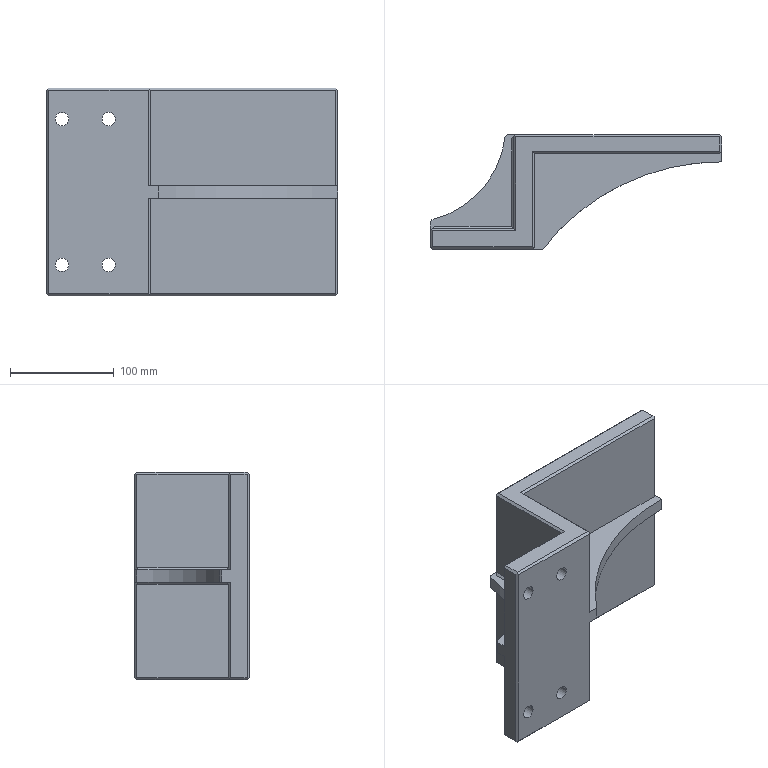Part | Creo | features CURVE 3, DATUM PLANE 3, CHAMFER 2, PROTRUSION 2, COORDINATE SYSTEM 1, CUT 1 | 1 solid | 60 faces | box 280 x 110 x 200 mm | volume 1505598 mm3 | plane 50 | cylinder 10 | commonest cylinder face diameters 13 x8 185.516 x1 436.19 x1